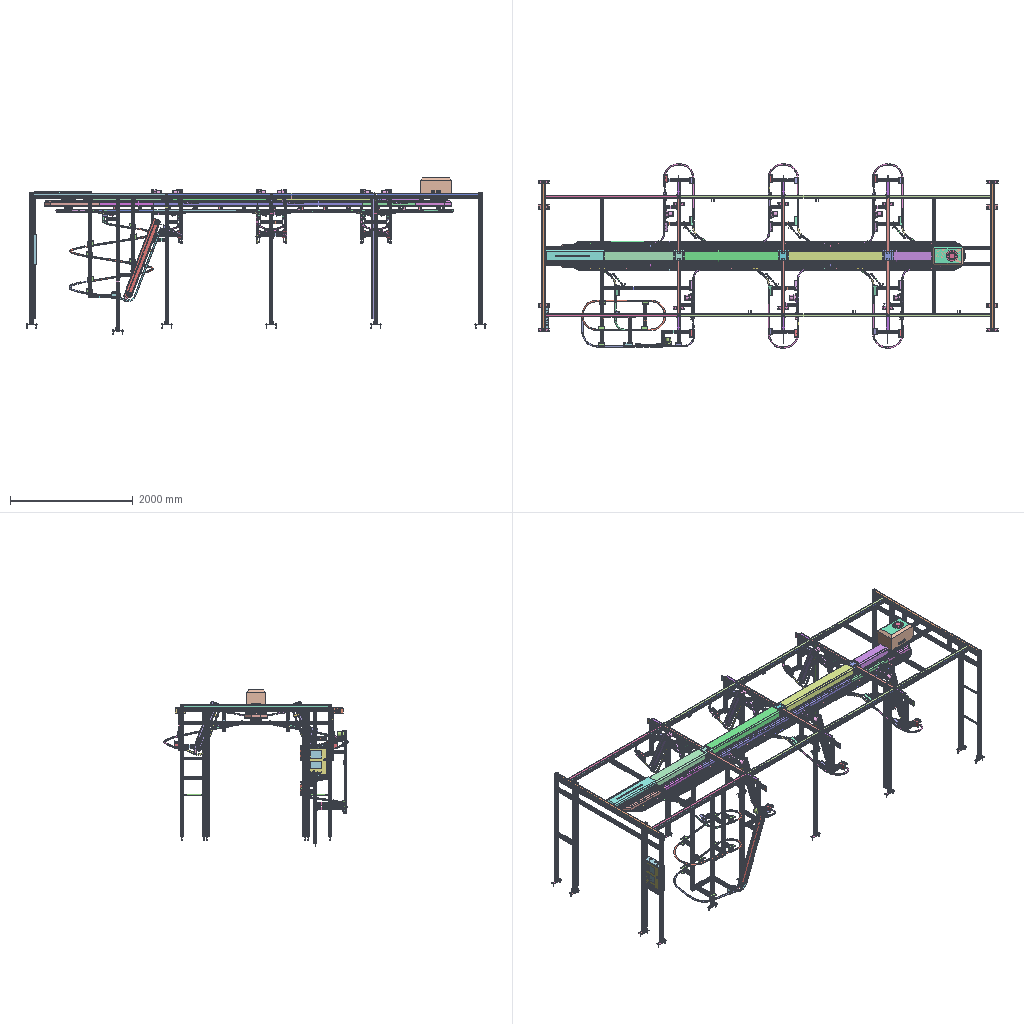Assembly | STEP file | 311 different items | 2384 placed | box 7480 x 3005 x 2565 mm
Parts list (item | name | quantity | parent item | size | volume):
1 | 101000005924 | x13 | in 31E-01008XJ12, 31E-01008XJ13, QG | 59.899 x 76.667 x 7.2 mm | 10614 mm3
2 | 101000005926 | x26 | in 31E-01008XJ12, 31E-01008XJ13, QG | 9 x 21.5 x 9 mm | 593.361 mm3
3 | 101000005927 | x13 | in 31E-01008XJ12, 31E-01008XJ13, QG | 88.898 x 18 x 18 mm | 15835 mm3
4 | 101000005928 | x38 | in 31E-01005JZ10, 31E-01008XJ12, 31E-01008XJ13, QG | 8.083 x 7 x 15.5 mm | 255.357 mm3
5 | 101000005929 | x13 | in 31E-01008XJ12, 31E-01008XJ13, QG | 30 x 13 x 13 mm | 1668 mm3
6 | 101000007578 | x12 | in BJX | 50 x 50 x 8.8 mm | 5573 mm3
7 | 101000007581 | x4 | in BJX | 56 x 32.4 x 56 mm | 27988 mm3
8 | 101000007583 | x6 | in 31E-01003CZ10 | - | -
9 | 101000007584 | x6 | in 31E-01005JZ10 | 28.845 x 44.401 x 156.082 mm | 37459 mm3
10 | 101000007593 | x13 | in 31E-01008XJ12, 31E-01008XJ13, QG | 18 x 17.5 x 69.846 mm | 7199 mm3
11 | 101000007596 | x6 | in 31E-01099TS10 | 14 x 75 x 75 mm | 33220 mm3
12 | 101000007597 | x1 | in 31E-01002TS11 | 14 x 75 x 75 mm | 33220 mm3
13 | 101000007604 | x14 | in 31E-01002TS11, 31E-01099TS10 | 2.7 x 25 x 25 mm | 785.143 mm3
14 | 101000007605 | x7 | in 31E-01002TS11, 31E-01099TS10 | 60 x 24.5 x 62.5 mm | 11628 mm3
15 | 101000007607 | x14 | in 31E-01002TS11, 31E-01099TS10 | 16 x 47 x 35 mm | 7077 mm3
16 | 101000007608 | x7 | in C, PJ | 73.608 x 80.551 x 25.4 mm | 31663 mm3
17 | 101000007616 | x1 | in HL-ED3000 | 3.719 x 7.9 x 15 mm | 372.862 mm3
18 | 101000007619 | x1 | in HL-ED3000 | 1000 x 2.5 x 152 mm | 378659 mm3
19 | 101000007619 [2] | x1 | in HL-ED3000 | 1000 x 2.5 x 152 mm | 378659 mm3
20 | 101000007619 [3] | x1 | in HL-ED3000 | 1000 x 2.5 x 152 mm | 378659 mm3
21 | 101000007619 [4] | x1 | in HL-ED3000 | 1000 x 2.5 x 152 mm | 378659 mm3
22 | 101000007619 [5] | x1 | in HL-ED3000 | 1000 x 2.5 x 152 mm | 378659 mm3
23 | 101000007619 [6] | x1 | in HL-ED3000 | 1000 x 2.5 x 152 mm | 378659 mm3
24 | 101000007620 | x1 | in HL-ED3000 | 225 x 129.5 x 170 mm | 152398 mm3
25 | 101000007620 [2] | x1 | in HL-ED3000 | 225 x 129.5 x 170 mm | 152398 mm3
26 | 101000007620 [3] | x1 | in HL-ED3000 | 225 x 129.5 x 170 mm | 152398 mm3
27 | 101000007695 | x8 | in 31E-01136WG10, 31E-01138WG10 | 77.497 x 4.891 x 169.241 mm | 7806 mm3
28 | 101000007696 | x4 | in 31E-01136WG10, 31E-01138WG10 | 13.848 x 4.891 x 29.9 mm | 904.543 mm3
29 | 101000007717 | x1 | in 003000000538 | 310 x 500 x 8 mm | 1181603 mm3
30 | 101000007723 | x7 | in 31E-01002TS11, 31E-01099TS10 | 3 x 160 x 90 mm | 38961 mm3
31 | 101000007733 | x1 | in 003000000538 | 153 x 296.456 x 296.456 mm | 689449 mm3
32 | 101000007742 | x1 | in 003000000538 | 68 x 72.975 x 68 mm | 70977 mm3
33 | 101000007750 | x7 | in 31E-01002TS11, 31E-01099TS10 | 34.924 x 12.5 x 12.5 mm | 1534 mm3
34 | 101000007761 | x6 | in 31E-01005JZ10 | 22.7 x 13 x 13 mm | 1455 mm3
35 | 101000007764 | x6 | in 31E-01003CZ10 | 16 x 16 x 30 mm | 4190 mm3
36 | 101000007768 | x1 | in 31E-01002TS11 | 17.508 x 2.203 x 8.5 mm | 152.771 mm3
37 | 101000007769 | x1 | in 31E-01002TS11 | 13.68 x 2.268 x 4.5 mm | 76.237 mm3
38 | 101000007773 | x1 | in HL-ED3000 | 505 x 315 x 290 mm | 663603 mm3
39 | 101000007774 | x1 | in HL-ED3000 | 245 x 56 x 950 mm | 323951 mm3
40 | 101000007777 | x8 | in C, HL-ED3000, PJ | 25.4 x 102.52 x 25.4 mm | 3984 mm3
41 | 101000007782 | x6 | in 31E-01005JZ10 | 63.5 x 78.9 x 12.709 mm | 13515 mm3
42 | 101000007783 | x6 | in 31E-01005JZ10 | 55 x 25.4 x 25.4 mm | 16233 mm3
43 | 101000007784 | x1 | in HL-ED3000 | 40 x 15 x 80 mm | 24612 mm3
44 | 101000007784 [2] | x1 | in HL-ED3000 | 40 x 15 x 80 mm | 24612 mm3
45 | 101000007784 [3] | x1 | in HL-ED3000 | 40 x 15 x 80 mm | 24612 mm3
46 | 101000007784 [4] | x1 | in HL-ED3000 | 40 x 15 x 80 mm | 24612 mm3
47 | 101000007785 | x1 | in 003000000538 | 34 x 34 x 10 mm | 8308 mm3
48 | 101000007788 | x1 | in 31E-M | 192 x 138 x 30 mm | 99773 mm3
49 | 101000007789 | x1 | in 003000000538 | 280 x 310 x 50 mm | 616529 mm3
50 | 101000007795 | x1 | in 31E-N | 192 x 138 x 5 mm | 83395 mm3
51 | 101000007811 | x13 | in 31E-01008XJ12, 31E-01008XJ13, QG | 37 x 22 x 10 mm | 1193 mm3
52 | 101000007812 | x2 | in SZLJK | 30.072 x 7.6 x 60 mm | 12718 mm3
53 | 101000007889 | x6 | in 31E-01003CZ10 | - | 638.551 mm3
54 | 101000008214 | x6 | in 31E-01003CZ10 | 21 x 17 x 115 mm | 12262 mm3
55 | 101000008215 | x6 | in 31E-01003CZ10 | 22.7 x 22.7 x 50 mm | 12976 mm3
56 | 101000008264 | x6 | in 31E-01003CZ10 | - | 2402 mm3
57 | 101000008265 | x6 | in 31E-01003CZ10 | 22.806 x 22.806 x 21.136 mm | 3240 mm3
58 | 102000006842 | x1 | in KJ | 350 x 500 x 106.8 mm | 412738 mm3
59 | 102000006924 | x20 | in 31E-01002TS11, 31E-01023QY13 | 25 x 14 x 5 mm | 1290 mm3
60 | 102000006924 [2] | x150 | in 31E-01021QY13, 31E-01024QY13, 31E-01026QY13, 31E-01028QY13, 31E-01099TS10, 51E-01147JG10, 51E-01148JG10, 51E-01149JG10, 51E-01198JG10 | 25 x 14 x 5 mm | 1290 mm3
61 | 102000006964 | x35 | in 31E-01002TS11, 31E-01099TS10 | 10 x 3.101 x 2 mm | 16.245 mm3
62 | 102000006971 | x14 | in 31E-01002TS11, 31E-01099TS10 | 8 x 3 x 16 mm | 158.982 mm3
63 | 102000006983 | x7 | in 31E-01002TS11, 31E-01099TS10 | 18 x 16 x 7 mm | 384 mm3
64 | 102000006984 | x7 | in 31E-01002TS11, 31E-01099TS10 | 2 x 2 x 100 mm | 314.159 mm3
65 | 102000006988 | x14 | in 31E-01002TS11, 31E-01099TS10 | 6 x 6 x 20 mm | 172.788 mm3
66 | 102000010051 | x6 | in 31E-01099TS10 | 80 x 80 x 152 mm | 650749 mm3
67 | 102000010056 | x1 | in 31E-01002TS11 | 80 x 80 x 152 mm | 651211 mm3
68 | 102000010058 | x1 | in 003000000538 | 199 x 195.5 x 352 mm | 5244332 mm3
69 | 102000010521 | x1 | in 31E-01002TS11 | 10 x 27.034 x 66.257 mm | 4509 mm3
70 | 102000010554 | x6 | in 31E-01005JZ10 | 157.5 x 18 x 18 mm | 33195 mm3
71 | 102000010555 | x1 | in HL-ED3000 | 572.24 x 75 x 75 mm | 1547367 mm3
72 | 103000006124 | x1 | in 31E-01002TS11 | 75 x 1341 x 10 mm | 174412 mm3
73 | 103000006127 | x6 | in 31E-01099TS10 | 75 x 826 x 10 mm | 108901 mm3
74 | 103000006174_M8×10 | x12 | in 51E-01144JG10, 51E-01145JG10 | 10 x 8 x 8 mm | 407.497 mm3
75 | 103000006185 | x12 | in 31E-01005JZ10 | 19 x 8.5 x 8.5 mm | 522.658 mm3
76 | 103000006194_ST5.5×22 | x14 | in 31E-01002TS11, 31E-01099TS10 | 28 x 11.2 x 11.2 mm | 709.482 mm3
77 | 103000006212 | x6 | in 31E-01005JZ10 | 8 x 4 x 4 mm | 88.508 mm3
78 | 103000006242_M3×16 | x14 | in 31E-01002TS11, 31E-01099TS10 | 18.351 x 5.6 x 5.6 mm | 155.702 mm3
79 | 103000006341_M10 | x6 | in 31E-01003CZ10 | 16 x 18.475 x 8.4 mm | 1391 mm3
80 | 103000006354_5×20 | x7 | in 31E-01002TS11, 31E-01099TS10 | 4.915 x 5 x 34.44 mm | 138.102 mm3
81 | 103000010384_M4×12 | x13 | in 31E-01008XJ12, 31E-01008XJ13, QG | 15.027 x 8 x 8 mm | 256.338 mm3
82 | 103000014839_5×20 | x12 | in 31E-01003CZ10 | 4.915 x 5 x 19.44 mm | 77.195 mm3
83 | 103000016257 | x30 | in 31E-01021QY13, 31E-01023QY13 | 80 x 16 x 16 mm | 6519 mm3
84 | 103000016289_10 | x6 | in 31E-01003CZ10 | 15.372 x 15.344 x 2.6 mm | 261.313 mm3
85 | 20301 | x1 | in 101000007916 | 860 x 310 x 6 mm | 1402017 mm3
86 | 20303 | x4 | in 101000007916 | 60 x 20 x 30 mm | 30649 mm3
87 | 20304 | x2 | in JL | 25 x 123 x 25 mm | 28266 mm3
88 | 20305 | x3 | in CHE40-500, JL | 24.5 x 60.843 x 62 mm | 24740 mm3
89 | 20307 | x1 | in ZJYD | 50 x 30 x 50 mm | 67161 mm3
90 | 20308 | x1 | in ZJYD | 45 x 30 x 8 mm | 9755 mm3
91 | 20309 | x2 | in 101000007916 | 20 x 20 x 580 mm | 182152 mm3
92 | 20310 | x4 | in 101000007916 | 60.5 x 51.5 x 20 mm | 29160 mm3
93 | 20312 | x1 | in ZJYD | 200 x 150 x 6 mm | 169265 mm3
94 | 20314 | x1 | in 101000007916 | 130 x 90 x 132 mm | 160571 mm3
95 | 20315 | x1 | in ZJYD | 40 x 26 x 50 mm | 20124 mm3
96 | 20316-1 | x1 | in 20316-0 | 178 x 43 x 43 mm | 148101 mm3
97 | 20316-2 | x1 | in 20316-0 | 80 x 80 x 14 mm | 53929 mm3
98 | 20318 | x1 | in ZJYD | 38.5 x 38.5 x 34 mm | 5928 mm3
99 | 20319 | x1 | in ZJYD | 71.5 x 71.5 x 31.5 mm | 12079 mm3
100 | 20322 | x1 | in ZJYD | 98 x 98 x 14 mm | 42100 mm3
101 | 31E-01000CC12 | x6 | in xian cao | 50 x 38.192 x 215 mm | 35398 mm3
102 | 31E-01000CC13 | x7 | in xian cao | 50 x 38.192 x 900 mm | 148176 mm3
103 | 31E-01000QY15 | x7 | in 31E-01002TS11, 31E-01099TS10 | 148.5 x 50 x 40 mm | 17043 mm3
104 | 31E-01001CC12 | x6 | in xian cao | 50 x 9.195 x 215 mm | 18858 mm3
105 | 31E-01001CC13 | x6 | in xian cao | 50 x 9.195 x 900 mm | 78943 mm3
106 | 31E-01001QY15 | x7 | in 31E-01002TS11, 31E-01099TS10 | 148.5 x 50 x 40 mm | 17812 mm3
107 | 31E-01002XJ15 | x8 | in 31E-01001XJ14, 31E-01001XJ15 | 69 x 89.5 x 114.175 mm | 78639 mm3
108 | 31E-01002XJ16 | x1 | in 31E-01001XJ16 | 71 x 89.5 x 159.175 mm | 114683 mm3
109 | 31E-01006QY25 | x4 | in KJ | 25.4 x 25.4 x 345 mm | 60669 mm3
110 | 31E-01009XJ12 | x6 | in 31E-01008XJ12 | 71 x 89.5 x 164.024 mm | 105161 mm3
111 | 31E-01009XJ13 | x6 | in 31E-01008XJ13 | 71 x 89.5 x 184.024 mm | 127988 mm3
112 | 31E-01010TS12 | x1 | in 31E-01002TS11 | 125 x 34 x 1360 mm | 828291 mm3
113 | 31E-01014QY25 | x12 | in 31E-01000ZD16, 31E-01014QY13 | 60 x 30.804 x 19.2 mm | 24408 mm3
114 | 31E-01017QY13 | x6 | in C, PJ | 22 x 22 x 110 mm | 10626 mm3
115 | 31E-01018XJ10 | x7 | in 31E-01006XJ11 | 69 x 89.5 x 119.024 mm | 78639 mm3
116 | 31E-01019QY13 | x6 | in C, PJ | 25.4 x 25.4 x 180 mm | 16074 mm3
117 | 31E-01020QY13 | x22 | in 31E-01021QY13 | 60 x 64.996 x 48 mm | 20307 mm3
118 | 31E-01020TS12 | x6 | in 31E-01099TS10 | 125 x 34 x 836 mm | 502303 mm3
119 | 31E-01022QY13 | x8 | in 31E-01023QY13 | 60 x 64.996 x 68 mm | 29020 mm3
120 | 31E-01024XJ10 | x6 | in 31E-02587BL10 | 69 x 89.5 x 174.024 mm | 118687 mm3
121 | 31E-01025QY13 | x3 | in 31E-01024QY13 | 48 x 3.5 x 105 mm | 16661 mm3
122 | 31E-01025QY25 | x2 | in xian cao | 50 x 38.192 x 2366 mm | 389538 mm3
123 | 31E-01026QY25 | x2 | in xian cao | 50 x 9.195 x 2366 mm | 207531 mm3
124 | 31E-01027QY13 | x2 | in 31E-01026QY13 | 48 x 3.5 x 160 mm | 25860 mm3
125 | 31E-01027QY25 | x2 | in xian cao | 50 x 38.192 x 2150 mm | 353976 mm3
126 | 31E-01028QY25 | x2 | in xian cao | 50 x 9.195 x 2150 mm | 188585 mm3
127 | 31E-01029QY13 | x1 | in 31E-01028QY13 | 60 x 64.996 x 25 mm | 10496 mm3
128 | 31E-01029QY25 | x4 | in xian cao | 50 x 38.192 x 2050 mm | 337512 mm3
129 | 31E-01030QY25 | x4 | in xian cao | 50 x 9.195 x 2050 mm | 179814 mm3
130 | 31E-01040QY25 | x14 | in 31E-01002TS11, 31E-01099TS10 | 21.5 x 9.856 x 28 mm | 3296 mm3
131 | 31E-01141WG10 | x1 | in C | 25.4 x 512.578 x 517.132 mm | 179398 mm3
132 | 31E-01142WG10 | x1 | in C | 783.998 x 763.4 x 302.048 mm | 329314 mm3
133 | 31E-01143WG10 | x3 | in C | 1031 x 498.4 x 311.784 mm | 326544 mm3
134 | 31E-01144WG10 | x1 | in C | 25.4 x 346.08 x 258.41 mm | 96204 mm3
135 | 31E-01145WG10 | x5 | in PJ | 512.979 x 777.537 x 350.463 mm | 265200 mm3
136 | 31E-01158WG10 | x6 | in 31E-01003CZ10 | 210.148 x 245.71 x 22 mm | 63051 mm3
137 | 410151501000_ST4.2×19 | x24 | in 31E-01008XJ12 | 8 x 8 x 22.035 mm | 343.522 mm3
138 | 410151501000_ST4.2×19 [2] | x28 | in 31E-01136WG10, 31E-01138WG10 | 8 x 8 x 22.035 mm | 343.522 mm3
139 | 46A-00003CC12 | x6 | in xian cao | 50 x 38.192 x 1650 mm | 271656 mm3
140 | 46A-00006CC11-1195mm | x1 | in 31E-01001ZD19 | 50 x 50 x 1195 mm | 702053 mm3
141 | 46A-00006CC11-1270mm | x1 | in 31E-01000ZD24 | 50 x 50 x 1270 mm | 746115 mm3
142 | 46A-00006CC11-1526mm | x2 | in 31E-01000DJ14, 31E-01000ZD15 | 50 x 50 x 1526 mm | 896513 mm3
143 | 46A-00006CC11-152mm | x26 | in 31E-01001XJ14, 31E-01006XJ11, 31E-01008XJ13, 31E-02587BL10 | 50 x 50 x 152 mm | 89299 mm3
144 | 46A-00006CC11-1610mm | x1 | in 31E-01000ZD22 | 50 x 50 x 1610 mm | 945863 mm3
145 | 46A-00006CC11-1650mm | x6 | in 31E-01000BZ17, 31E-01001BZ17, 31E-01006BZ17 | 50 x 50 x 1650 mm | 969108 mm3
146 | 46A-00006CC11-165mm | x2 | in 31E-01000DJ15 | 50 x 50 x 165 mm | 96936 mm3
147 | 46A-00006CC11-187mm | x6 | in 31E-01000BZ16 | 50 x 50 x 187 mm | 109861 mm3
148 | 46A-00006CC11-1880mm | x2 | in 31E-01000DJ13, 31E-01000ZD14 | 50 x 50 x 1880 mm | 1104486 mm3
149 | 46A-00006CC11-200mm | x1 | in 31E-01001BZ15 | 50 x 50 x 200 mm | 117498 mm3
150 | 46A-00006CC11-2050mm | x6 | in 31E-01000BZ11, 31E-01000ZD21 | 50 x 50 x 2050 mm | 1204359 mm3
151 | 46A-00006CC11-210mm | x1 | in 31E-01000BZ10 | 50 x 50 x 210 mm | 123373 mm3
152 | 46A-00006CC11-2150mm | x1 | in 31E-01000ZD13 | 50 x 50 x 2150 mm | 1262854 mm3
153 | 46A-00006CC11-2150mm-2 | x6 | in 31E-01000DJ12, 31E-01001ZD13, 31E-01001ZD21, Tensioning end outer frame end column | 50 x 50 x 2150 mm | 1263109 mm3
154 | 46A-00006CC11-220mm | x1 | in 31E-01000DJ16 | 50 x 50 x 220 mm | 129248 mm3
155 | 46A-00006CC11-240mm | x1 | in 31E-01000ZD27 | 50 x 50 x 240 mm | 140998 mm3
156 | 46A-00006CC11-2410mm | x3 | in 31E-01000ZD19, 31E-01001BZ10 | 50 x 50 x 2410 mm | 1415857 mm3
157 | 46A-00006CC11-275mm | x6 | in 31E-02586BL10 | 50 x 50 x 275 mm | 161560 mm3
158 | 46A-00006CC11-330mm | x13 | in 31E-01000BZ14, 31E-01045QY25, 31E-02518BL10 | 50 x 50 x 330 mm | 193872 mm3
159 | 46A-00006CC11-350mm | x6 | in 31E-01000ZD17 | 50 x 50 x 350 mm | 205622 mm3
160 | 46A-00006CC11-400mm | x1 | in 31E-01000BZ15 | 50 x 50 x 400 mm | 234997 mm3
161 | 46A-00006CC11-417mm | x2 | in 31E-01001XJ15, 31E-01001XJ16 | 50 x 50 x 417 mm | 244984 mm3
162 | 46A-00006CC11-845mm | x1 | in 31E-04412BL10 | 50 x 50 x 845 mm | 496431 mm3
163 | 46A-00006CC11-905 | x2 | in 31E-01000DJ10 | 50 x 50 x 905 mm | 531426 mm3
164 | 46A-00008CC12 | x6 | in xian cao | 50 x 9.195 x 1650 mm | 144728 mm3
165 | 46A-00010CC11-2040mm | x4 | in 31E-01000DJ17, Tensioning end outer frame double column | 50 x 70 x 2040 mm | 1443284 mm3
166 | 46A-00010CC11-2366mm | x2 | in 31E-01000DJ11, Tensioning outer frame crossbeam assembly | 70 x 50 x 2366 mm | 1673926 mm3
167 | 46A-01000LM15_Default<As Machined> | x26 | in 31E-01008XJ12, 31E-01008XJ13, QG | 6.634 x 7.66 x 6 mm | 155.687 mm3
168 | 46A-01001LM15_Default<As Machined> | x26 | in 31E-01008XJ12, 31E-01008XJ13, QG | 9.238 x 8 x 7.2 mm | 261.678 mm3
169 | 46A-01001LS14_Default<As Machined> | x28 | in 31E-01002TS11, 31E-01099TS10 | 14 x 8.9 x 8.9 mm | 333.383 mm3
170 | 46A-01001LS15_Default<As Machined> | x13 | in 31E-01008XJ12, 31E-01008XJ13, QG | 23.057 x 8 x 8 mm | 332.138 mm3
171 | 46A-01002LM15_Default<As Machined> | x7 | in 31E-01002TS11, 31E-01099TS10 | 11.547 x 10 x 8.5 mm | 503.163 mm3
172 | 46A-01002LM1_Default<As Machined> | x12 | in 31E-M, 31E-N | 11.547 x 10 x 8.5 mm | 503.163 mm3
173 | 46A-01005CC13 | x4 | in 51E-01144JG10 | 10.8 x 35.7 x 80 mm | 20059 mm3
174 | 46A-01006CC13 | x2 | in 51E-01145JG10 | 22 x 9.7 x 140 mm | 22186 mm3
175 | 46A-01009CC13 | x275 | in 31E-01000BZ11, 31E-01000BZ17, 31E-01000DJ10, 31E-01000DJ11, 31E-01000DJ12, 31E-01000DJ13, 31E-01000DJ14, 31E-01000DJ17, 31E-01000ZD13, 31E-01000ZD14, 31E-01000ZD19, 31E-01000ZD21, 31E-01000ZD22, 31E-01000ZD24, 31E-01000ZD27, 31E-01001BZ10, 31E-01001BZ17, 31E-01001ZD13, 31E-01001ZD19, 31E-01001ZD21, 31E-01006BZ17, 31E-01045QY25, 31E-02518BL10, 31E-02586BL10, 31E-04412BL10, 31E-04413BL10, Tensioning end outer frame double column, Tensioning end outer frame end column, Tensioning outer frame crossbeam assembly | 21.5 x 60 x 60 mm | 15069 mm3
176 | 46A-01010CC13 | x12 | in SZGD, SZLJK | 61.971 x 28 x 61.971 mm | 69920 mm3
177 | 46B-01002ZX30 | x6 | in 31E-01005JZ10 | 44.236 x 35.015 x 50.429 mm | 13200 mm3
178 | 46B-01003ZX30 | x6 | in 31E-01005JZ10 | 43.778 x 27.592 x 52.956 mm | 12356 mm3
179 | 46D-01016ZX15 | x6 | in 31E-01099TS10 | 10 x 27.034 x 66.257 mm | 4509 mm3
180 | 51E-01017SL10 | x1 | in ZHP | 173.954 x 20.1 x 100 mm | 57654 mm3
181 | 51E-01018SL10 | x1 | in ZHP | 173.954 x 20.1 x 100 mm | 57563 mm3
182 | 51E-01019SL10 | x1 | in ZHP | 173.954 x 20.1 x 100 mm | 57557 mm3
183 | 51E-01020SL10 | x1 | in ZHP | 173.954 x 20.1 x 100 mm | 57557 mm3
184 | 51E-01021SL10 | x1 | in ZHP | 173.954 x 20.1 x 100 mm | 57536 mm3
185 | 51E-01022SL10 | x1 | in ZHP | 173.954 x 20.1 x 100 mm | 57540 mm3
186 | 51E-01143JG10 | x2 | in 31E-1, 31E-2 | 62 x 90 x 2980 mm | 2562098 mm3
187 | 51E-01155JG10 | x1 | in HL-ED3000 | 62 x 90 x 2631 mm | 2262137 mm3
188 | 51E-01158JG10 | x1 | in HL-ED3000 | 62 x 90 x 2631 mm | 2262137 mm3
189 | 51E-01159JG10 | x1 | in HL-ED3000 | 19.8 x 19.8 x 100 mm | 11184 mm3
190 | 51E-01159JG10 [2] | x1 | in HL-ED3000 | 19.8 x 19.8 x 100 mm | 11184 mm3
191 | 51E-01159JG10 [3] | x1 | in HL-ED3000 | 19.8 x 19.8 x 100 mm | 11184 mm3
192 | 51E-01159JG10 [4] | x1 | in HL-ED3000 | 19.8 x 19.8 x 100 mm | 11184 mm3
193 | 51E-01159JG10 [5] | x1 | in HL-ED3000 | 19.8 x 19.8 x 100 mm | 11184 mm3
194 | 51E-01159JG10 [6] | x1 | in HL-ED3000 | 19.8 x 19.8 x 100 mm | 11184 mm3
195 | 51E-01163JG10 | x1 | in HL-ED3000 | 1000 x 25.4 x 25.4 mm | 190883 mm3
196 | 51E-01163JG10 [2] | x1 | in HL-ED3000 | 1000 x 25.4 x 25.4 mm | 190883 mm3
197 | 51E-01164JG10 | x1 | in HL-ED3000 | 22 x 22 x 300 mm | 53721 mm3
198 | 51E-01164JG10 [2] | x1 | in HL-ED3000 | 22 x 22 x 300 mm | 53721 mm3
199 | 51E-01178JG10 | x1 | in HL-ED3000 | 62 x 90 x 30 mm | 25669 mm3
200 | 51E-01179JG10 | x1 | in HL-ED3000 | 62 x 90 x 30 mm | 25669 mm3
201 | 51E-01200JG10 | x1 | in HL-ED3000 | 67.801 x 18.48 x 1520 mm | 173727 mm3
202 | 51E-01200JG10 [2] | x1 | in HL-ED3000 | 67.801 x 18.48 x 1520 mm | 173727 mm3
203 | 51E-01201JG10 | x1 | in HL-ED3000 | 67.801 x 18.48 x 1700 mm | 194300 mm3
204 | 51E-01201JG10 [2] | x1 | in HL-ED3000 | 67.801 x 18.48 x 1700 mm | 194300 mm3
205 | 51E-01201JG10 [3] | x1 | in HL-ED3000 | 67.801 x 18.48 x 1700 mm | 194300 mm3
206 | 51E-01201JG10 [4] | x1 | in HL-ED3000 | 67.801 x 18.48 x 1700 mm | 194300 mm3
207 | 51E-01202JG10 | x1 | in HL-ED3000 | 67.801 x 18.48 x 225 mm | 25716 mm3
208 | 51E-01202JG10 [2] | x1 | in HL-ED3000 | 67.801 x 18.48 x 225 mm | 25716 mm3
209 | 51E-01203JG10 | x1 | in HL-ED3000 | 600 x 355 x 5 mm | 492755 mm3
210 | 51E-01203JG10 [2] | x1 | in HL-ED3000 | 600 x 355 x 5 mm | 492755 mm3
211 | 51E-01204JG10 | x1 | in HL-ED3000 | 2100 x 355 x 5 mm | 1842144 mm3
212 | 51E-01204JG10 [2] | x1 | in HL-ED3000 | 2100 x 355 x 5 mm | 1842144 mm3
213 | 51E-01205JG10 | x1 | in HL-ED3000 | 1800 x 355 x 5 mm | 1579291 mm3
214 | 51E-01206JG10 | x1 | in HL-ED3000 | 367.304 x 82.9 x 577.652 mm | 277740 mm3
215 | 51E-01207JG10 | x1 | in HL-ED3000 | 367.304 x 82.9 x 899.652 mm | 410628 mm3
216 | 51E-01208JG10 | x1 | in HL-ED3000 | 65 x 82.9 x 870 mm | 179523 mm3
217 | 51E-01208JG10 [2] | x1 | in HL-ED3000 | 65 x 82.9 x 870 mm | 179523 mm3
218 | 51E-01208JG10 [3] | x1 | in HL-ED3000 | 65 x 82.9 x 870 mm | 179523 mm3
219 | 51E-01208JG10 [4] | x1 | in HL-ED3000 | 65 x 82.9 x 870 mm | 179523 mm3
220 | 51E-01209JG10 | x3 | in HL-ED3000 | 65 x 82.9 x 1700 mm | 350793 mm3
221 | 51E-01209JG10 [2] | x1 | in HL-ED3000 | 65 x 82.9 x 1700 mm | 350793 mm3
222 | 51E-01211JG10 | x1 | in 31E-01136WG10 | 483.4 x 541.7 x 25.4 mm | 262302 mm3
223 | 51E-01212JG10 | x1 | in 31E-01138WG10 | 483.4 x 491.7 x 25.4 mm | 222157 mm3
224 | 51E-01213JG10 | x2 | in 31E-M, 31E-N | 154.2 x 68 x 40 mm | 48152 mm3
225 | 51E-01214JG10 | x2 | in 31E-M, 31E-N | 154.2 x 68 x 40 mm | 48290 mm3
226 | 51E-01215JG10 | x2 | in 31E-M, 31E-N | 154.2 x 68 x 40 mm | 48290 mm3
227 | 51E-01219JG10 | x1 | in HL-ED3000 | 67.801 x 18.48 x 1550 mm | 173193 mm3
228 | 51E-01220JG10 | x1 | in HL-ED3000 | 67.801 x 18.48 x 1550 mm | 173193 mm3
229 | 51E-01221JG10 | x1 | in HL-ED3000 | 225 x 127 x 1570 mm | 1681663 mm3
230 | 51E-01221JG10 [2] | x1 | in HL-ED3000 | 225 x 127 x 1570 mm | 1681663 mm3
231 | 51E-01222JG10 | x1 | in HL-ED3000 | 225 x 127 x 650 mm | 696230 mm3
232 | 51E-01223JG10 | x1 | in HL-ED3000 | 225 x 127 x 1150 mm | 1231792 mm3
233 | DZZC_730mm | x5 | in 31E-04413BL10 | 50 x 50 x 675 mm | 396557 mm3
234 | DZZC_905mm | x2 | in 31E-01000ZD16 | 50 x 50 x 905 mm | 530917 mm3
235 | Drive sprocket | x1 | in ZJYD | 70 x 296.646 x 296.646 mm | 579512 mm3
236 | GB/T6184-20001 type all-metal hex lock nut M16 | x6 | in JL | 23.219 x 26.75 x 15.2 mm | 3899 mm3
237 | PN_0004_Default<As Machined> | x13 | in 31E-01008XJ12, 31E-01008XJ13, QG | 9.88 x 9.88 x 1.6 mm | 64.212 mm3
238 | PN_0004_Default<As Machined> [2] | x30 | in 31E-01005JZ10 | 9.88 x 9.88 x 1.6 mm | 64.212 mm3
239 | PN_0004_Default<As Machined> [3] | x12 | in 31E-M, 31E-N | 9.88 x 9.88 x 1.6 mm | 64.212 mm3
240 | PN_0005_Default<As Machined> | x26 | in 31E-01008XJ12, 31E-01008XJ13, QG | 14.75 x 9.5 x 9.5 mm | 350.853 mm3
241 | PN_0006_Default<As Machined> | x28 | in 31E-01002TS11, 31E-01099TS10 | 16 x 5.2 x 5.2 mm | 125.378 mm3
242 | PN_0007_Default<As Machined> | x21 | in 31E-01002TS11, 31E-01099TS10 | 16 x 16 x 1.6 mm | 219.912 mm3
243 | PN_0008_Default<As Machined> | x14 | in 31E-01002TS11, 31E-01099TS10 | 24 x 13 x 13 mm | 1618 mm3
244 | PN_0009_Default<As Machined> | x35 | in 31E-01002TS11, 31E-01099TS10 | 12.88 x 12.88 x 2.1 mm | 143.97 mm3
245 | PN_0009_Default<As Machined> [2] | x1 | in 003000000538 | 12.88 x 12.88 x 2.1 mm | 143.97 mm3
246 | PN_0010_Default<As Machined> | x2 | in 101000007602 | 19 x 6 x 19 mm | 1190 mm3
247 | PN_0011_Default<As Machined> | x28 | in 31E-01002TS11, 31E-01099TS10 | 22 x 13 x 13 mm | 1485 mm3
248 | PN_0012_Default<As Machined> | x14 | in 31E-01002TS11, 31E-01099TS10 | 6.351 x 5.5 x 2.4 mm | 46.625 mm3
249 | PN_0014_Default<As Machined> | x7 | in 31E-01002TS11, 31E-01099TS10 | 24 x 24 x 2 mm | 793.943 mm3
250 | PN_0015_Default<As Machined> | x14 | in 31E-01002TS11, 31E-01099TS10 | 5 x 5 x 0.8 mm | 8.148 mm3
251 | PN_0016_Default<As Machined> | x2 | in 31E-01002TS11 | 10 x 3.5 x 3.5 mm | 35.87 mm3
252 | PN_0018_Default<As Machined> | x1 | in 31E-01002TS11 | 1294 x 25.4 x 262.259 mm | 292213 mm3
253 | PN_0019_Default<As Machined> | x18 | in 31E-01005JZ10 | 10.681 x 11.495 x 6.499 mm | 404.351 mm3
254 | PN_0020_Default<As Machined> | x12 | in 31E-01005JZ10 | 10 x 10 x 1 mm | 54.782 mm3
255 | PN_0021_Default<As Machined> | x12 | in 31E-01005JZ10 | 10.045 x 10.045 x 31.074 mm | 1111 mm3
256 | PN_0022_Default<As Machined> | x12 | in 31E-01005JZ10 | 8 x 8 x 1.3 mm | 34.299 mm3
257 | PN_0022_Default<As Machined> [2] | x6 | in 51E-01149JG10 | 8 x 8 x 1.3 mm | 34.299 mm3
258 | PN_0023_Default<As Machined> | x6 | in 31E-01005JZ10 | 12 x 12 x 1.6 mm | 126.217 mm3
259 | PN_0023_Default<As Machined> [2] | x12 | in 31E-M, 31E-N | 12 x 12 x 1.6 mm | 126.217 mm3
260 | PN_0024_Default<As Machined> | x6 | in 31E-01005JZ10 | 25 x 28 x 2.5 mm | 1599 mm3
261 | PN_0025_Default<As Machined> | x6 | in 31E-01005JZ10 | 18.993 x 19.771 x 10.003 mm | 799.735 mm3
262 | PN_0026_Default<As Machined> | x6 | in 31E-01005JZ10 | 25 x 37.475 x 110 mm | 10034 mm3
263 | PN_0027_Default<As Machined> | x6 | in 31E-01005JZ10 | 382.183 x 95.469 x 27.278 mm | 74724 mm3
264 | PN_0028_Default<As Machined> | x12 | in 101000007665-1 | 19 x 6 x 19 mm | 1190 mm3
265 | PN_0029_Default<As Machined> | x6 | in 31E-01099TS10 | 380.934 x 25.4 x 797.47 mm | 220981 mm3
266 | PN_0030_Default<As Machined> | x82 | in 31E-01021QY13, 31E-01023QY13, 31E-01024QY13, 31E-01026QY13, 31E-01028QY13 | 16.4 x 14 x 14 mm | 997.771 mm3
267 | PN_0031_Default<As Machined> | x26 | in 51E-01147JG10, 51E-01198JG10 | 20 x 13 x 13 mm | 1442 mm3
268 | PN_0032_Default<As Machined> | x6 | in 51E-01198JG10 | 28 x 13 x 13 mm | 1794 mm3
269 | PN_0033_Default<As Machined> | x6 | in 51E-01198JG10 | 24 x 24 x 10 mm | 3970 mm3
270 | PN_0034_Default<As Machined> | x28 | in 51E-01148JG10, 51E-01149JG10 | 20 x 13 x 13 mm | 1442 mm3
271 | PN_0035_Default<As Machined> | x6 | in 51E-01149JG10 | 9.632 x 9.5 x 9.5 mm | 311.012 mm3
272 | PN_0037_Default<As Machined> | x12 | in 31E-M, 31E-N | 26 x 10 x 10 mm | 888.028 mm3
273 | PN_0038_Default<As Machined> | x2 | in 31E-M | 16.25 x 52 x 52 mm | 18571 mm3
274 | PN_0039_Default<As Machined> | x1 | in HL-ED3000 | 25.4 x 2940 x 25.4 mm | 584472 mm3
275 | PN_0039_Default<As Machined> [2] | x1 | in HL-ED3000 | 25.4 x 2940 x 25.4 mm | 584472 mm3
276 | PN_0040_Default<As Machined> | x1 | in 003000000538 | 43 x 13 x 13 mm | 2467 mm3
277 | PN_0041_Default<As Machined> | x1 | in 003000000538 | 54 x 58.103 x 2 mm | 1371 mm3
278 | PN_0042_Default<As Machined> | x2 | in 003000000538 | 34.641 x 34.641 x 8 mm | 4654 mm3
279 | PN_0043_Default<As Machined> | x3 | in 003000000538 | 28 x 13 x 13 mm | 1794 mm3
280 | PN_0044_Default<As Machined> | x1 | in 003000000538 | 20 x 90 x 90 mm | 65138 mm3
281 | PN_0045_Default<As Machined> | x1 | in 003000000538 | 96 x 100.912 x 2.5 mm | 4237 mm3
282 | PN_0046_Default<As Machined> | x1 | in HL-ED3000 | 25.4 x 1683 x 25.4 mm | 334580 mm3
283 | PN_0046_Default<As Machined> [2] | x1 | in HL-ED3000 | 25.4 x 1683 x 25.4 mm | 334580 mm3
284 | V00-000000445 | x10 | in 51E-01147JG10 | 60 x 64.996 x 25 mm | 10496 mm3
285 | V00-000000446 | x5 | in 51E-01147JG10 | 26 x 12 x 155 mm | 17713 mm3
286 | V00-000000447 | x22 | in 51E-01148JG10 | 157.7 x 151.5 x 40 mm | 68710 mm3
287 | V00-000000448 | x6 | in 51E-01149JG10 | 157.7 x 151.5 x 40 mm | 68668 mm3
288 | V00-000000449 | x6 | in 51E-01149JG10 | 84.272 x 12.5 x 20 mm | 3695 mm3
289 | V00-000000450 | x6 | in 51E-01198JG10 | 60 x 64.996 x 25 mm | 9956 mm3
290 | V00-000000453 | x2 | in 101000007682 | 254.244 x 18.951 x 254.244 mm | 49463 mm3
291 | V00-000000454 | x2 | in 101000007682 | 234.244 x 18.951 x 254.244 mm | 49218 mm3
292 | V00-000000627 | x1 | in 101000007602 | 16 x 75 x 75 mm | 34582 mm3
293 | V00-000000634 | x6 | in 31E-01008XJ12 | 50 x 50 x 152 mm | 89299 mm3
294 | V00-000000855 | x6 | in 101000007665-1 | 16 x 75 x 75 mm | 34582 mm3
295 | ZDDQ | x2 | in ZJYD | 45.173 x 54.71 x 1 mm | 912.343 mm3
296 | ZDDQ-M20 | x1 | in ZJYD | 38 x 38 x 1 mm | 382.357 mm3
297 | _CHE40-500_c1 | x48 | in CHE40-500 | 23 x 10.3 x 16.04 mm | 895.191 mm3
298 | _CHE40-500_c2 | x49 | in CHE40-500 | 24.4 x 11.7 x 10.95 mm | 1210 mm3
299 | _Headless pin DIN 913 - M5x8 | x3 | in PLNY20 | 8 x 5 x 5 mm | 135.796 mm3
300 | _Headless pin DIN 913 - M6x8 | x6 | in PLNY30 | 8 x 6 x 6 mm | 188.543 mm3
301 | _JMDBB63-400(0)_BODY | x1 | in JMDBB63-400(0_0_0) | 495 x 70 x 70 mm | 538960 mm3
302 | _JMDBB63-400_ROD | x1 | in JMDBB63-400(0_0_0) | 492.5 x 63 x 63 mm | 139467 mm3
303 | _JNTC40 | x1 | in CHE40-500 | 23 x 10.3 x 17.55 mm | 1033 mm3
304 | _LH-RRING-C-INT-S-32 | x8 | in LHBB20 | 1.2 x 32.2 x 33.7 mm | 309.422 mm3
305 | _LHBB20-1_b | x4 | in LHBB20 | 54 x 41 x 50 mm | 55289 mm3
306 | _LMU-N20 | x4 | in LHBB20 | 42 x 32 x 32 mm | 20321 mm3
307 | _MSW8 | x20 | in 31E-01014QY13 | 8 x 8 x 8 mm | 320.313 mm3
308 | _NT-05(63)_JMB_NUT | x1 | in JMDBB63-400(0_0_0) | 11 x 31.177 x 27 mm | 4550 mm3
309 | _PLNY20x | x1 | in PLNY20 | 10 x 32 x 32 mm | 4486 mm3
310 | _PLNY30x | x2 | in PLNY30 | 12 x 45 x 45 mm | 10207 mm3
311 | _SPWF16 | x6 | in JL | 1.8 x 30 x 30 mm | 863.783 mm3